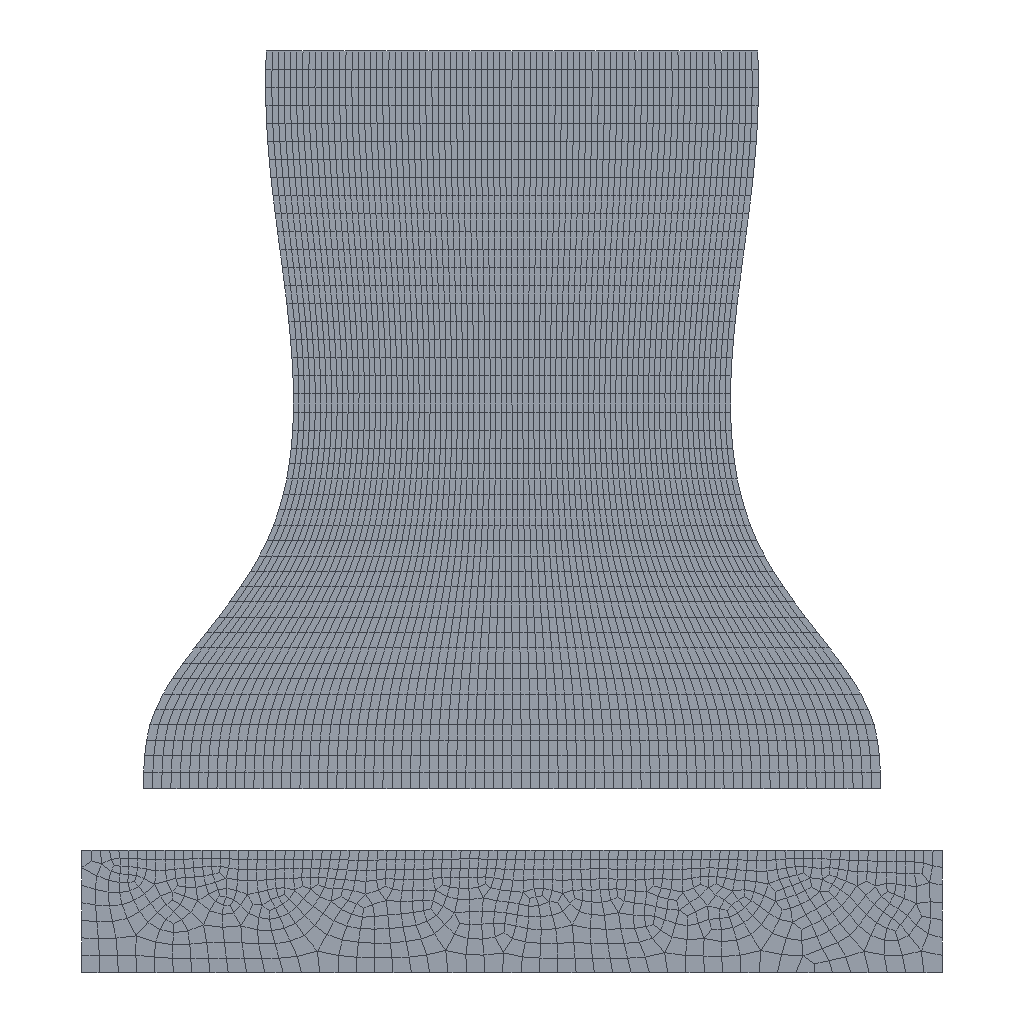Simulation study | abaqus
Set-up summary:
category,name,step,type,value,unit,region
solver,abaqus
solver,version,,,Abaqus/Standard 2020
units,not stated in the deck,,not stated
analysis,deck,,static,static
load_step,Step-1,Step-1,static
load_step,Step-3,Step-3,static
load_step,requested,,,2
mesh,nodes,,,4490
mesh,elements,,,4287
element_type,CPS4R,,plane,4287
load,load commands in deck,,count,2
bc,support commands in deck,,count,5
material,MIRROR,,in results
material,PDMS,,in results
material,SILICONRUBBER,,in results
material,TPU1,,in results
material,TPU10,,in results
material,TPU11,,in results
material,TPU2,,in results
material,TPU3,,in results
material,TPU4,,in results
material,TPU5,,in results
material,TPU6,,in results
material,TPU7,,in results
material,TPU8,,in results
material,TPU9,,in results
check,setup vs results,,match,"per instance, exact: element labels, types and connectivity; labels of the nodes the elements use; coordinates of those nodes at SINGLE_PRECISION in 2 of 2 instance(s)"
Abaqus input file, long lists of numbers shortened:
*Heading
** Job name: Job-3 Model name: Model-1-Copy-Copy
** Generated by: Abaqus/CAE 2020
*Preprint, echo=NO, model=NO, history=NO, contact=NO
**
** PARTS
**
*Part, name=Mirror
*Node
      1,   137.021,           0.
      2,   131.064,           0.
** (843 more lines like these left out)
*Element, type=CPS4R
  1,  33,  31, 494,  72
  2,  72, 494, 455,  73
** (765 more lines like these left out)
*Nset, nset=_PickedSet3, internal, generate
   1,  845,    1
*Elset, elset=_PickedSet3, internal, generate
   1,  767,    1
*Elset, elset=_Surf-Mirror_S2, internal
  13,  19,  26,  33,  46,  60,  66,  72,  78,  84,  91,  95, 109, 115, 121, 127
 134, 141, 148, 154, 160, 164, 177, 183, 189, 195, 283, 344, 347, 349, 351, 353
** (2 more lines like these left out)
*Elset, elset=_Surf-Mirror_S4, internal
  40,  53, 102, 171, 284, 285, 287, 289, 290, 292, 293, 295, 296, 297, 299, 301
 303, 305, 307, 309, 310, 311, 313, 315, 317, 319, 321, 323, 325, 327, 329, 331
** (1 more lines like these left out)
*Elset, elset=_Surf-Mirror_S1, internal
 200, 383
*Elset, elset=_Surf-Mirror_S3, internal
 341,
*Surface, type=ELEMENT, name=Surf-Mirror
_Surf-Mirror_S2, S2
_Surf-Mirror_S4, S4
_Surf-Mirror_S1, S1
_Surf-Mirror_S3, S3
** Section: t1
*Solid Section, elset=_PickedSet3, material=TPU1
,
*End Part
**
*Part, name=mushroom
*Node
      1,  -35.915,   15.373
      2,   35.915,   15.373
** (3643 more lines like these left out)
*Element, type=CPS4R
   1,    1,   27, 1118,  226
   2,   27,   28, 1119, 1118
** (3518 more lines like these left out)
*Nset, nset=FORCE
 3,
*Nset, nset=BOTTOM
  21,  22, 874, 875, 876, 877, 878, 879, 880, 881, 882, 883, 884, 885, 886, 887
 888, 889, 890, 891, 892, 893, 894, 895, 896, 897, 898, 899, 900, 901, 902, 903
** (4 more lines like these left out)
*Elset, elset=BOTTOM, generate
 2961,  3040,     1
*Nset, nset=Set-23
   19,   20,   21,   22,  794,  795,  796,  797,  798,  799,  800,  801,  802,  803,  804,  805
  806,  807,  808,  809,  810,  811,  812,  813,  814,  815,  816,  817,  818,  819,  820,  821
** (14 more lines like these left out)
*Elset, elset=Set-23, generate
 2881,  3040,     1
*Nset, nset=Set-24
   19,   20,   25,   26,  794,  795,  796,  797,  798,  799,  800,  801,  802,  803,  804,  805
  806,  807,  808,  809,  810,  811,  812,  813,  814,  815,  816,  817,  818,  819,  820,  821
** (14 more lines like these left out)
*Elset, elset=Set-24, generate
 3201,  3360,     1
*Nset, nset=Set-25
   23,   24,   25,   26,  955,  956,  957,  958,  959,  960,  961,  962,  963,  964,  965,  966
  967,  968,  969,  970,  971,  972,  973,  974,  975,  976,  977,  978,  979,  980,  981,  982
** (14 more lines like these left out)
*Elset, elset=Set-25, generate
 3361,  3520,     1
*Nset, nset=Set-26
   17,   18,   23,   24,  713,  714,  715,  716,  717,  718,  719,  720,  721,  722,  723,  724
  725,  726,  727,  728,  729,  730,  731,  732,  733,  734,  735,  736,  737,  738,  739,  740
** (14 more lines like these left out)
*Elset, elset=Set-26, generate
 3041,  3200,     1
*Nset, nset=Set-27
   15,   16,   17,   18,  633,  634,  635,  636,  637,  638,  639,  640,  641,  642,  643,  644
  645,  646,  647,  648,  649,  650,  651,  652,  653,  654,  655,  656,  657,  658,  659,  660
** (14 more lines like these left out)
*Elset, elset=Set-27, generate
 2721,  2880,     1
*Nset, nset=Set-28
   13,   14,   15,   16,  551,  552,  553,  554,  555,  556,  557,  558,  559,  560,  561,  562
  563,  564,  565,  566,  567,  568,  569,  570,  571,  572,  573,  574,  575,  576,  577,  578
** (14 more lines like these left out)
*Elset, elset=Set-28, generate
 2561,  2720,     1
*Nset, nset=Set-29
   11,   12,   13,   14,  471,  472,  473,  474,  475,  476,  477,  478,  479,  480,  481,  482
  483,  484,  485,  486,  487,  488,  489,  490,  491,  492,  493,  494,  495,  496,  497,  498
** (14 more lines like these left out)
*Elset, elset=Set-29, generate
 2401,  2560,     1
*Nset, nset=Set-30
    9,   10,   11,   12,  389,  390,  391,  392,  393,  394,  395,  396,  397,  398,  399,  400
  401,  402,  403,  404,  405,  406,  407,  408,  409,  410,  411,  412,  413,  414,  415,  416
** (14 more lines like these left out)
*Elset, elset=Set-30, generate
 2241,  2400,     1
*Nset, nset=Set-31
    7,    8,    9,   10,  309,  310,  311,  312,  313,  314,  315,  316,  317,  318,  319,  320
  321,  322,  323,  324,  325,  326,  327,  328,  329,  330,  331,  332,  333,  334,  335,  336
** (14 more lines like these left out)
*Elset, elset=Set-31, generate
 2081,  2240,     1
*Nset, nset=Set-32
    5,    6,    7,    8,  227,  228,  229,  230,  231,  232,  233,  234,  235,  236,  237,  238
  239,  240,  241,  242,  243,  244,  245,  246,  247,  248,  249,  250,  251,  252,  253,  254
** (14 more lines like these left out)
*Elset, elset=Set-32, generate
 1921,  2080,     1
*Nset, nset=Set-33
    1,    2,    5,    6,   27,   28,   29,   30,   31,   32,   33,   34,   35,   36,   37,   38
   39,   40,   41,   42,   43,   44,   45,   46,   47,   48,   49,   50,   51,   52,   53,   54
** (14 more lines like these left out)
*Elset, elset=Set-33, generate
 1761,  1920,     1
*Nset, nset=Set-34
    1,    2,    3,    4,   27,   28,   29,   30,   31,   32,   33,   34,   35,   36,   37,   38
   39,   40,   41,   42,   43,   44,   45,   46,   47,   48,   49,   50,   51,   52,   53,   54
** (115 more lines like these left out)
*Elset, elset=Set-34, generate
    1,  1760,     1
*Elset, elset=_Surf-BOTTOM_S3, internal, generate
 2961,  3040,     1
*Surface, type=ELEMENT, name=Surf-BOTTOM
_Surf-BOTTOM_S3, S3
** Section: t11
*Solid Section, elset=Set-34, material=TPU11
,
** Section: t11
*Solid Section, elset=Set-33, material=TPU11
,
** Section: t10
*Solid Section, elset=Set-32, material=TPU10
,
** Section: t9
*Solid Section, elset=Set-31, material=TPU9
,
** Section: t8
*Solid Section, elset=Set-30, material=TPU8
,
** Section: t7
*Solid Section, elset=Set-29, material=TPU7
,
** Section: t6
*Solid Section, elset=Set-28, material=TPU6
,
** Section: t5
*Solid Section, elset=Set-27, material=TPU5
,
** Section: t1
*Solid Section, elset=Set-23, material=TPU1
,
** Section: t4
*Solid Section, elset=Set-26, material=TPU4
,
** Section: t2
*Solid Section, elset=Set-24, material=TPU2
,
** Section: t3
*Solid Section, elset=Set-25, material=TPU3
,
*End Part
**
**
** ASSEMBLY
**
*Assembly, name=Assembly
**
*Instance, name=Mirror-1, part=Mirror
        -70.,         -70.,           0.
*End Instance
**
*Instance, name=mushroom-1, part=mushroom
*End Instance
**
*Node
      1,         -70.,         -50.,           0.
*Node
      2,          70.,         -50.,           0.
*Nset, nset=Set-2, instance=Mirror-1
   1,   2,   3,   4,   5,   6,   7,   8,   9,  10,  11,  12,  13,  14,  15,  16
  17,  18,  19,  20,  21,  22,  23,  24,  25,  26,  27,  28,  29,  30,  31,  32
** (1 more lines like these left out)
*Elset, elset=Set-2, instance=Mirror-1
   1,   8,   9,  15,  21,  22,  28,  35,  36,  42,  48,  49,  55,  56,  62,  68
  69,  74,  80,  86,  87,  93,  97,  98, 104, 105, 117, 123, 129, 130, 136, 143
** (1 more lines like these left out)
*Nset, nset=Set-4, instance=mushroom-1
   3,   4, 127, 128, 129, 130, 131, 132, 133, 134, 135, 136, 137, 138, 139, 140
 141, 142, 143, 144, 145, 146, 147, 148, 149, 150, 151, 152, 153, 154, 155, 156
** (4 more lines like these left out)
*Elset, elset=Set-4, instance=mushroom-1, generate
 1681,  1760,     1
*End Assembly
*Amplitude, name=Amp-1
             0.,              0.,              1.,              1.
**
** MATERIALS
**
*Material, name=Mirror
*Density
 9.3e-07,
*Elastic
10000., 0.5
*Material, name=PDMS
*Density
 9.3e-07,
*Hyperelastic, neo hooke
 0.662, 0.255
*Material, name=SiliconRubber
*Density
 9.3e-07,
*Hyperelastic, mooney-rivlin
 0.111, 0.039, 0.001
*Material, name=TPU1
*Density
 9.3e-07,
*Elastic
20., 0.4
*Material, name=TPU2
*Density
 9.3e-07,
*Elastic
19., 0.4
*Material, name=TPU3
*Density
 9.3e-07,
*Elastic
18., 0.4
*Material, name=TPU4
*Density
 9.3e-07,
*Elastic
17., 0.4
*Material, name=TPU5
*Density
 9.3e-07,
*Elastic
16., 0.4
*Material, name=TPU6
*Density
 9.3e-07,
*Elastic
15., 0.4
*Material, name=TPU7
*Density
 9.3e-07,
*Elastic
14., 0.4
*Material, name=TPU8
*Density
 9.3e-07,
*Elastic
13., 0.4
*Material, name=TPU9
*Density
 9.3e-07,
*Elastic
12., 0.4
*Material, name=TPU10
*Density
 9.3e-07,
*Elastic
11., 0.4
*Material, name=TPU11
*Density
 9.3e-07,
*Elastic
10., 0.4
**
** INTERACTION PROPERTIES
**
*Surface Interaction, name=INTPROP-1
1.,
*Friction, slip tolerance=0.005
0.,
*Surface Behavior, pressure-overclosure=HARD
*Surface Interaction, name=INTPROP-COH
1.,
*Cohesive Behavior, REPEATED CONTACTS, eligibility=CURRENT CONTACTS
 0.25, 0.25, 0.25
*Damage Initiation, criterion=MAXS
 0.05, 0.05, 0.05
*Damage Evolution, type=DISPLACEMENT, softening=EXPONENTIAL
 0.205,2.
*Damage Stabilization
0.01
**
** BOUNDARY CONDITIONS
**
** Name: BC-2 Type: 对称/反对称/完全固定
*Boundary
Set-2, ENCASTRE
**
** INTERACTIONS
**
** Interaction: Int-1
*Contact
*Contact Inclusions, ALL EXTERIOR
*Contact Property Assignment
 ,  , INTPROP-1
** ----------------------------------------------------------------
**
** STEP: Step-1
**
*Step, name=Step-1, nlgeom=YES
*Static, stabilize=0.0002, allsdtol=0.05, continue=NO
0.01, 1., 1e-05, 0.1
**
** BOUNDARY CONDITIONS
**
** Name: [REDACTED] : Displacement/rotation angle
*Boundary, amplitude=Amp-1
Set-4, 1, 1
Set-4, 2, 2, -22.9
Set-4, 6, 6
**
** OUTPUT REQUESTS
**
*Restart, write, frequency=0
**
** FIELD OUTPUT: F-Output-1
**
*Output, field
*Node Output
CF, RF, RM, RT, U, V
*Element Output, directions=YES
E, LE, MISES, MISESONLY, PE, PEEQ, PEMAG, S, SSAVG
*Contact Output
CDISP, CSTRESS
**
** HISTORY OUTPUT: H-Output-1
**
*Output, history, variable=PRESELECT
*End Step
** ----------------------------------------------------------------
**
** STEP: Step-3
**
*Step, name=Step-3, nlgeom=YES, inc=10000000
*Static, stabilize=0.0002, allsdtol=0.05, continue=NO
0.001, 1., 1e-10, 0.01
**
** BOUNDARY CONDITIONS
**
** Name: [REDACTED] : Displacement/rotation angle
*Boundary, amplitude=Amp-1
Set-4, 2, 2, 30.
**
** OUTPUT REQUESTS
**
*Restart, write, frequency=0
**
** FIELD OUTPUT: F-Output-1
**
*Output, field
*Node Output
CF, RF, RM, RT, U, V
*Element Output, directions=YES
E, LE, MISES, MISESONLY, PE, PEEQ, PEMAG, S, SSAVG
*Contact Output
CDISP, CSTRESS
**
** HISTORY OUTPUT: H-Output-1
**
*Output, history, variable=PRESELECT
*End Step
Results summary:
result,step,,completed,increments=19 time=1.0/1.0
result,step,,completed,increments=106 time=1.0/1.0
result,analysis,,,static
result,last_loadstep,,,2
result,primary field,,,U
result,reaction total,,FX,0.0,model units
result,reaction total,,FY,0.0,model units
result,reaction total,,FZ,0.0,model units